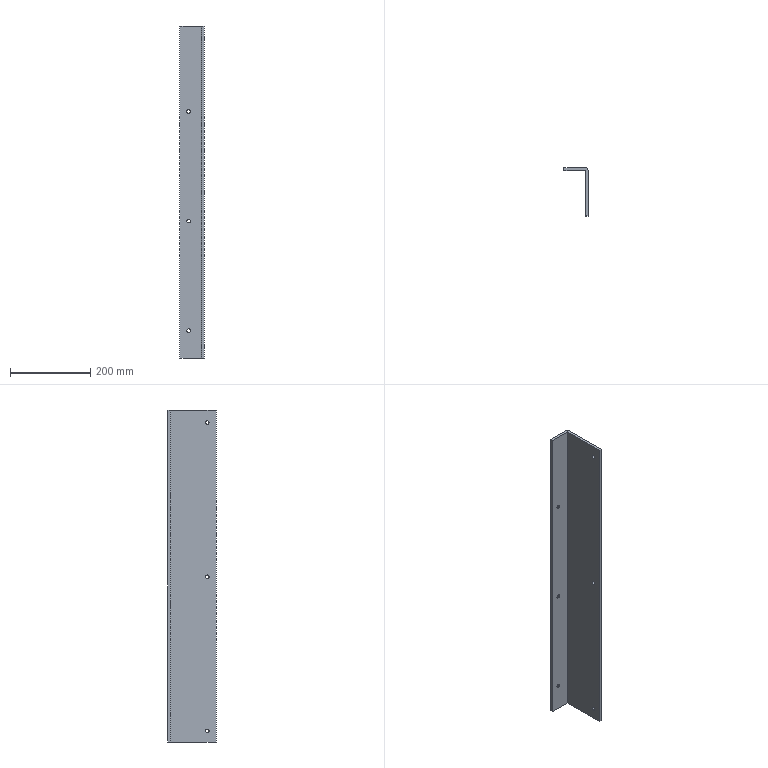Part | SolidWorks | features BaseBody 1 | 1 solid | 28 faces | box 60 x 120 x 827 mm | volume 851995 mm3 | cylinder 14 | plane 8 | cone 6 | commonest cylinder face diameters 9 x12 1.473 x1 13.473 x1
STEP:
#1=CARTESIAN_POINT('',(-6.,22.,800.));
#2=VERTEX_POINT('',#1);
#3=CARTESIAN_POINT('',(-6.,22.,791.));
#4=VERTEX_POINT('',#3);
#5=CARTESIAN_POINT('',(-6.,22.,795.5));
#6=DIRECTION('',(1.,0.,0.));
#7=DIRECTION('',(0.,0.,-1.));
#8=AXIS2_PLACEMENT_3D('',#5,#6,#7);
#9=CIRCLE('',#8,4.5);
#10=EDGE_CURVE('',#2,#4,#9,.T.);
#11=ORIENTED_EDGE('',*,*,#10,.F.);
#12=CARTESIAN_POINT('',(0.,22.,800.));
#13=VERTEX_POINT('',#12);
#14=CARTESIAN_POINT('',(-60.,22.,800.));
#15=DIRECTION('',(1.,0.,0.));
#16=VECTOR('',#15,1000.);
#17=LINE('',#14,#16);
#18=EDGE_CURVE('',#2,#13,#17,.T.);
#19=ORIENTED_EDGE('',*,*,#18,.T.);
#20=CARTESIAN_POINT('',(0.,22.,791.));
#21=VERTEX_POINT('',#20);
#22=CARTESIAN_POINT('',(0.,22.,795.5));
#23=DIRECTION('',(1.,0.,0.));
#24=DIRECTION('',(0.,0.,-1.));
#25=AXIS2_PLACEMENT_3D('',#22,#23,#24);
#26=CIRCLE('',#25,4.5);
#27=EDGE_CURVE('',#13,#21,#26,.T.);
#28=ORIENTED_EDGE('',*,*,#27,.T.);
#29=CARTESIAN_POINT('',(-60.,22.,791.));
#30=DIRECTION('',(1.,0.,0.));
#31=VECTOR('',#30,1000.);
#32=LINE('',#29,#31);
#33=EDGE_CURVE('',#4,#21,#32,.T.);
#34=ORIENTED_EDGE('',*,*,#33,.F.);
#35=EDGE_LOOP('',(#11,#19,#28,#34));
#36=FACE_OUTER_BOUND('',#35,.T.);
#37=CARTESIAN_POINT('',(-60.,22.,795.5));
#38=DIRECTION('',(1.,0.,0.));
#39=DIRECTION('',(0.,0.,-1.));
#40=AXIS2_PLACEMENT_3D('',#37,#38,#39);
#41=CYLINDRICAL_SURFACE('',#40,4.5);
#42=ADVANCED_FACE('',(#36),#41,.F.);
#43=CARTESIAN_POINT('',(-6.,22.,416.));
#44=VERTEX_POINT('',#43);
#45=CARTESIAN_POINT('',(-6.,22.,407.));
#46=VERTEX_POINT('',#45);
#47=CARTESIAN_POINT('',(-6.,22.,411.5));
#48=DIRECTION('',(1.,0.,0.));
#49=DIRECTION('',(0.,0.,-1.));
#50=AXIS2_PLACEMENT_3D('',#47,#48,#49);
#51=CIRCLE('',#50,4.5);
#52=EDGE_CURVE('',#44,#46,#51,.T.);
#53=ORIENTED_EDGE('',*,*,#52,.F.);
#54=CARTESIAN_POINT('',(0.,22.,416.));
#55=VERTEX_POINT('',#54);
#56=CARTESIAN_POINT('',(-60.,22.,416.));
#57=DIRECTION('',(1.,0.,0.));
#58=VECTOR('',#57,1000.);
#59=LINE('',#56,#58);
#60=EDGE_CURVE('',#44,#55,#59,.T.);
#61=ORIENTED_EDGE('',*,*,#60,.T.);
#62=CARTESIAN_POINT('',(0.,22.,407.));
#63=VERTEX_POINT('',#62);
#64=CARTESIAN_POINT('',(0.,22.,411.5));
#65=DIRECTION('',(1.,0.,0.));
#66=DIRECTION('',(0.,0.,-1.));
#67=AXIS2_PLACEMENT_3D('',#64,#65,#66);
#68=CIRCLE('',#67,4.5);
#69=EDGE_CURVE('',#55,#63,#68,.T.);
#70=ORIENTED_EDGE('',*,*,#69,.T.);
#71=CARTESIAN_POINT('',(-60.,22.,407.));
#72=DIRECTION('',(1.,0.,0.));
#73=VECTOR('',#72,1000.);
#74=LINE('',#71,#73);
#75=EDGE_CURVE('',#46,#63,#74,.T.);
#76=ORIENTED_EDGE('',*,*,#75,.F.);
#77=EDGE_LOOP('',(#53,#61,#70,#76));
#78=FACE_OUTER_BOUND('',#77,.T.);
#79=CARTESIAN_POINT('',(-60.,22.,411.5));
#80=DIRECTION('',(1.,0.,0.));
#81=DIRECTION('',(0.,0.,-1.));
#82=AXIS2_PLACEMENT_3D('',#79,#80,#81);
#83=CYLINDRICAL_SURFACE('',#82,4.5);
#84=ADVANCED_FACE('',(#78),#83,.F.);
#85=CARTESIAN_POINT('',(-6.,22.,32.));
#86=VERTEX_POINT('',#85);
#87=CARTESIAN_POINT('',(-6.,22.,23.));
#88=VERTEX_POINT('',#87);
#89=CARTESIAN_POINT('',(-6.,22.,27.5));
#90=DIRECTION('',(1.,0.,0.));
#91=DIRECTION('',(0.,0.,-1.));
#92=AXIS2_PLACEMENT_3D('',#89,#90,#91);
#93=CIRCLE('',#92,4.5);
#94=EDGE_CURVE('',#86,#88,#93,.T.);
#95=ORIENTED_EDGE('',*,*,#94,.F.);
#96=CARTESIAN_POINT('',(0.,22.,32.));
#97=VERTEX_POINT('',#96);
#98=CARTESIAN_POINT('',(-60.,22.,32.));
#99=DIRECTION('',(1.,0.,0.));
#100=VECTOR('',#99,1000.);
#101=LINE('',#98,#100);
#102=EDGE_CURVE('',#86,#97,#101,.T.);
#103=ORIENTED_EDGE('',*,*,#102,.T.);
#104=CARTESIAN_POINT('',(0.,22.,23.));
#105=VERTEX_POINT('',#104);
#106=CARTESIAN_POINT('',(0.,22.,27.5));
#107=DIRECTION('',(1.,0.,0.));
#108=DIRECTION('',(0.,0.,-1.));
#109=AXIS2_PLACEMENT_3D('',#106,#107,#108);
#110=CIRCLE('',#109,4.5);
#111=EDGE_CURVE('',#97,#105,#110,.T.);
#112=ORIENTED_EDGE('',*,*,#111,.T.);
#113=CARTESIAN_POINT('',(-60.,22.,23.));
#114=DIRECTION('',(1.,0.,0.));
#115=VECTOR('',#114,1000.);
#116=LINE('',#113,#115);
#117=EDGE_CURVE('',#88,#105,#116,.T.);
#118=ORIENTED_EDGE('',*,*,#117,.F.);
#119=EDGE_LOOP('',(#95,#103,#112,#118));
#120=FACE_OUTER_BOUND('',#119,.T.);
#121=CARTESIAN_POINT('',(-60.,22.,27.5));
#122=DIRECTION('',(1.,0.,0.));
#123=DIRECTION('',(0.,0.,-1.));
#124=AXIS2_PLACEMENT_3D('',#121,#122,#123);
#125=CYLINDRICAL_SURFACE('',#124,4.5);
#126=ADVANCED_FACE('',(#120),#125,.F.);
#127=CARTESIAN_POINT('',(-34.,115.5,68.));
#128=VERTEX_POINT('',#127);
#129=CARTESIAN_POINT('',(-38.5,115.5,63.5));
#130=VERTEX_POINT('',#129);
#131=CARTESIAN_POINT('',(-38.5,115.5,68.));
#132=DIRECTION('',(0.,1.,0.));
#133=DIRECTION('',(0.,0.,1.));
#134=AXIS2_PLACEMENT_3D('',#131,#132,#133);
#135=CIRCLE('',#134,4.5);
#136=EDGE_CURVE('',#128,#130,#135,.T.);
#137=ORIENTED_EDGE('',*,*,#136,.F.);
#138=CARTESIAN_POINT('',(-29.5,120.,68.));
#139=VERTEX_POINT('',#138);
#140=CARTESIAN_POINT('',(-29.5,120.,68.));
#141=DIRECTION('',(0.7071,0.7071,0.));
#142=VECTOR('',#141,1000.);
#143=LINE('',#140,#142);
#144=EDGE_CURVE('',#128,#139,#143,.T.);
#145=ORIENTED_EDGE('',*,*,#144,.T.);
#146=CARTESIAN_POINT('',(-47.5,120.,68.));
#147=VERTEX_POINT('',#146);
#148=CARTESIAN_POINT('',(-38.5,120.,68.));
#149=DIRECTION('',(0.,1.,0.));
#150=DIRECTION('',(-1.,0.,0.));
#151=AXIS2_PLACEMENT_3D('',#148,#149,#150);
#152=CIRCLE('',#151,9.);
#153=EDGE_CURVE('',#139,#147,#152,.T.);
#154=ORIENTED_EDGE('',*,*,#153,.T.);
#155=CARTESIAN_POINT('',(-43.,115.5,68.));
#156=VERTEX_POINT('',#155);
#157=CARTESIAN_POINT('',(-47.5,120.,68.));
#158=DIRECTION('',(-0.7071,0.7071,0.));
#159=VECTOR('',#158,1000.);
#160=LINE('',#157,#159);
#161=EDGE_CURVE('',#156,#147,#160,.T.);
#162=ORIENTED_EDGE('',*,*,#161,.F.);
#163=CARTESIAN_POINT('',(-38.5,115.5,68.));
#164=DIRECTION('',(0.,1.,0.));
#165=DIRECTION('',(0.,0.,1.));
#166=AXIS2_PLACEMENT_3D('',#163,#164,#165);
#167=CIRCLE('',#166,4.5);
#168=EDGE_CURVE('',#130,#156,#167,.T.);
#169=ORIENTED_EDGE('',*,*,#168,.F.);
#170=EDGE_LOOP('',(#137,#145,#154,#162,#169));
#171=FACE_OUTER_BOUND('',#170,.T.);
#172=CARTESIAN_POINT('',(-38.5,120.,68.));
#173=DIRECTION('',(0.,1.,0.));
#174=DIRECTION('',(-1.,0.,0.));
#175=AXIS2_PLACEMENT_3D('',#172,#173,#174);
#176=CONICAL_SURFACE('',#175,9.,0.7854);
#177=ADVANCED_FACE('',(#171),#176,.F.);
#178=CARTESIAN_POINT('',(-34.,115.5,614.));
#179=VERTEX_POINT('',#178);
#180=CARTESIAN_POINT('',(-38.5,115.5,609.5));
#181=VERTEX_POINT('',#180);
#182=CARTESIAN_POINT('',(-38.5,115.5,614.));
#183=DIRECTION('',(0.,1.,0.));
#184=DIRECTION('',(0.,0.,1.));
#185=AXIS2_PLACEMENT_3D('',#182,#183,#184);
#186=CIRCLE('',#185,4.5);
#187=EDGE_CURVE('',#179,#181,#186,.T.);
#188=ORIENTED_EDGE('',*,*,#187,.F.);
#189=CARTESIAN_POINT('',(-29.5,120.,614.));
#190=VERTEX_POINT('',#189);
#191=CARTESIAN_POINT('',(-29.5,120.,614.));
#192=DIRECTION('',(0.7071,0.7071,0.));
#193=VECTOR('',#192,1000.);
#194=LINE('',#191,#193);
#195=EDGE_CURVE('',#179,#190,#194,.T.);
#196=ORIENTED_EDGE('',*,*,#195,.T.);
#197=CARTESIAN_POINT('',(-47.5,120.,614.));
#198=VERTEX_POINT('',#197);
#199=CARTESIAN_POINT('',(-38.5,120.,614.));
#200=DIRECTION('',(0.,1.,0.));
#201=DIRECTION('',(-1.,0.,0.));
#202=AXIS2_PLACEMENT_3D('',#199,#200,#201);
#203=CIRCLE('',#202,9.);
#204=EDGE_CURVE('',#190,#198,#203,.T.);
#205=ORIENTED_EDGE('',*,*,#204,.T.);
#206=CARTESIAN_POINT('',(-43.,115.5,614.));
#207=VERTEX_POINT('',#206);
#208=CARTESIAN_POINT('',(-47.5,120.,614.));
#209=DIRECTION('',(-0.7071,0.7071,0.));
#210=VECTOR('',#209,1000.);
#211=LINE('',#208,#210);
#212=EDGE_CURVE('',#207,#198,#211,.T.);
#213=ORIENTED_EDGE('',*,*,#212,.F.);
#214=CARTESIAN_POINT('',(-38.5,115.5,614.));
#215=DIRECTION('',(0.,1.,0.));
#216=DIRECTION('',(0.,0.,1.));
#217=AXIS2_PLACEMENT_3D('',#214,#215,#216);
#218=CIRCLE('',#217,4.5);
#219=EDGE_CURVE('',#181,#207,#218,.T.);
#220=ORIENTED_EDGE('',*,*,#219,.F.);
#221=EDGE_LOOP('',(#188,#196,#205,#213,#220));
#222=FACE_OUTER_BOUND('',#221,.T.);
#223=CARTESIAN_POINT('',(-38.5,120.,614.));
#224=DIRECTION('',(0.,1.,0.));
#225=DIRECTION('',(-1.,0.,0.));
#226=AXIS2_PLACEMENT_3D('',#223,#224,#225);
#227=CONICAL_SURFACE('',#226,9.,0.7854);
#228=ADVANCED_FACE('',(#222),#227,.F.);
#229=CARTESIAN_POINT('',(-34.,115.5,341.));
#230=VERTEX_POINT('',#229);
#231=CARTESIAN_POINT('',(-38.5,115.5,336.5));
#232=VERTEX_POINT('',#231);
#233=CARTESIAN_POINT('',(-38.5,115.5,341.));
#234=DIRECTION('',(0.,1.,0.));
#235=DIRECTION('',(0.,0.,1.));
#236=AXIS2_PLACEMENT_3D('',#233,#234,#235);
#237=CIRCLE('',#236,4.5);
#238=EDGE_CURVE('',#230,#232,#237,.T.);
#239=ORIENTED_EDGE('',*,*,#238,.F.);
#240=CARTESIAN_POINT('',(-29.5,120.,341.));
#241=VERTEX_POINT('',#240);
#242=CARTESIAN_POINT('',(-29.5,120.,341.));
#243=DIRECTION('',(0.7071,0.7071,0.));
#244=VECTOR('',#243,1000.);
#245=LINE('',#242,#244);
#246=EDGE_CURVE('',#230,#241,#245,.T.);
#247=ORIENTED_EDGE('',*,*,#246,.T.);
#248=CARTESIAN_POINT('',(-47.5,120.,341.));
#249=VERTEX_POINT('',#248);
#250=CARTESIAN_POINT('',(-38.5,120.,341.));
#251=DIRECTION('',(0.,1.,0.));
#252=DIRECTION('',(-1.,0.,0.));
#253=AXIS2_PLACEMENT_3D('',#250,#251,#252);
#254=CIRCLE('',#253,9.);
#255=EDGE_CURVE('',#241,#249,#254,.T.);
#256=ORIENTED_EDGE('',*,*,#255,.T.);
#257=CARTESIAN_POINT('',(-43.,115.5,341.));
#258=VERTEX_POINT('',#257);
#259=CARTESIAN_POINT('',(-47.5,120.,341.));
#260=DIRECTION('',(-0.7071,0.7071,0.));
#261=VECTOR('',#260,1000.);
#262=LINE('',#259,#261);
#263=EDGE_CURVE('',#258,#249,#262,.T.);
#264=ORIENTED_EDGE('',*,*,#263,.F.);
#265=CARTESIAN_POINT('',(-38.5,115.5,341.));
#266=DIRECTION('',(0.,1.,0.));
#267=DIRECTION('',(0.,0.,1.));
#268=AXIS2_PLACEMENT_3D('',#265,#266,#267);
#269=CIRCLE('',#268,4.5);
#270=EDGE_CURVE('',#232,#258,#269,.T.);
#271=ORIENTED_EDGE('',*,*,#270,.F.);
#272=EDGE_LOOP('',(#239,#247,#256,#264,#271));
#273=FACE_OUTER_BOUND('',#272,.T.);
#274=CARTESIAN_POINT('',(-38.5,120.,341.));
#275=DIRECTION('',(0.,1.,0.));
#276=DIRECTION('',(-1.,0.,0.));
#277=AXIS2_PLACEMENT_3D('',#274,#275,#276);
#278=CONICAL_SURFACE('',#277,9.,0.7854);
#279=ADVANCED_FACE('',(#273),#278,.F.);
#280=CARTESIAN_POINT('',(-38.5,114.,63.5));
#281=VERTEX_POINT('',#280);
#282=CARTESIAN_POINT('',(-38.5,114.,72.5));
#283=VERTEX_POINT('',#282);
#284=CARTESIAN_POINT('',(-38.5,114.,68.));
#285=DIRECTION('',(0.,1.,0.));
#286=DIRECTION('',(0.,0.,1.));
#287=AXIS2_PLACEMENT_3D('',#284,#285,#286);
#288=CIRCLE('',#287,4.5);
#289=EDGE_CURVE('',#281,#283,#288,.T.);
#290=ORIENTED_EDGE('',*,*,#289,.F.);
#291=CARTESIAN_POINT('',(-38.5,120.,63.5));
#292=DIRECTION('',(0.,1.,0.));
#293=VECTOR('',#292,1000.);
#294=LINE('',#291,#293);
#295=EDGE_CURVE('',#281,#130,#294,.T.);
#296=ORIENTED_EDGE('',*,*,#295,.T.);
#297=ORIENTED_EDGE('',*,*,#168,.T.);
#298=CARTESIAN_POINT('',(-38.5,115.5,72.5));
#299=VERTEX_POINT('',#298);
#300=CARTESIAN_POINT('',(-38.5,115.5,68.));
#301=DIRECTION('',(0.,1.,0.));
#302=DIRECTION('',(0.,0.,1.));
#303=AXIS2_PLACEMENT_3D('',#300,#301,#302);
#304=CIRCLE('',#303,4.5);
#305=EDGE_CURVE('',#156,#299,#304,.T.);
#306=ORIENTED_EDGE('',*,*,#305,.T.);
#307=CARTESIAN_POINT('',(-38.5,120.,72.5));
#308=DIRECTION('',(0.,1.,0.));
#309=VECTOR('',#308,1000.);
#310=LINE('',#307,#309);
#311=EDGE_CURVE('',#283,#299,#310,.T.);
#312=ORIENTED_EDGE('',*,*,#311,.F.);
#313=EDGE_LOOP('',(#290,#296,#297,#306,#312));
#314=FACE_OUTER_BOUND('',#313,.T.);
#315=CARTESIAN_POINT('',(-38.5,120.,68.));
#316=DIRECTION('',(0.,1.,0.));
#317=DIRECTION('',(0.,0.,1.));
#318=AXIS2_PLACEMENT_3D('',#315,#316,#317);
#319=CYLINDRICAL_SURFACE('',#318,4.5);
#320=ADVANCED_FACE('',(#314),#319,.F.);
#321=CARTESIAN_POINT('',(-38.5,114.,609.5));
#322=VERTEX_POINT('',#321);
#323=CARTESIAN_POINT('',(-38.5,114.,618.5));
#324=VERTEX_POINT('',#323);
#325=CARTESIAN_POINT('',(-38.5,114.,614.));
#326=DIRECTION('',(0.,1.,0.));
#327=DIRECTION('',(0.,0.,1.));
#328=AXIS2_PLACEMENT_3D('',#325,#326,#327);
#329=CIRCLE('',#328,4.5);
#330=EDGE_CURVE('',#322,#324,#329,.T.);
#331=ORIENTED_EDGE('',*,*,#330,.F.);
#332=CARTESIAN_POINT('',(-38.5,120.,609.5));
#333=DIRECTION('',(0.,1.,0.));
#334=VECTOR('',#333,1000.);
#335=LINE('',#332,#334);
#336=EDGE_CURVE('',#322,#181,#335,.T.);
#337=ORIENTED_EDGE('',*,*,#336,.T.);
#338=ORIENTED_EDGE('',*,*,#219,.T.);
#339=CARTESIAN_POINT('',(-38.5,115.5,618.5));
#340=VERTEX_POINT('',#339);
#341=CARTESIAN_POINT('',(-38.5,115.5,614.));
#342=DIRECTION('',(0.,1.,0.));
#343=DIRECTION('',(0.,0.,1.));
#344=AXIS2_PLACEMENT_3D('',#341,#342,#343);
#345=CIRCLE('',#344,4.5);
#346=EDGE_CURVE('',#207,#340,#345,.T.);
#347=ORIENTED_EDGE('',*,*,#346,.T.);
#348=CARTESIAN_POINT('',(-38.5,120.,618.5));
#349=DIRECTION('',(0.,1.,0.));
#350=VECTOR('',#349,1000.);
#351=LINE('',#348,#350);
#352=EDGE_CURVE('',#324,#340,#351,.T.);
#353=ORIENTED_EDGE('',*,*,#352,.F.);
#354=EDGE_LOOP('',(#331,#337,#338,#347,#353));
#355=FACE_OUTER_BOUND('',#354,.T.);
#356=CARTESIAN_POINT('',(-38.5,120.,614.));
#357=DIRECTION('',(0.,1.,0.));
#358=DIRECTION('',(0.,0.,1.));
#359=AXIS2_PLACEMENT_3D('',#356,#357,#358);
#360=CYLINDRICAL_SURFACE('',#359,4.5);
#361=ADVANCED_FACE('',(#355),#360,.F.);
#362=CARTESIAN_POINT('',(-38.5,114.,336.5));
#363=VERTEX_POINT('',#362);
#364=CARTESIAN_POINT('',(-38.5,114.,345.5));
#365=VERTEX_POINT('',#364);
#366=CARTESIAN_POINT('',(-38.5,114.,341.));
#367=DIRECTION('',(0.,1.,0.));
#368=DIRECTION('',(0.,0.,1.));
#369=AXIS2_PLACEMENT_3D('',#366,#367,#368);
#370=CIRCLE('',#369,4.5);
#371=EDGE_CURVE('',#363,#365,#370,.T.);
#372=ORIENTED_EDGE('',*,*,#371,.F.);
#373=CARTESIAN_POINT('',(-38.5,120.,336.5));
#374=DIRECTION('',(0.,1.,0.));
#375=VECTOR('',#374,1000.);
#376=LINE('',#373,#375);
#377=EDGE_CURVE('',#363,#232,#376,.T.);
#378=ORIENTED_EDGE('',*,*,#377,.T.);
#379=ORIENTED_EDGE('',*,*,#270,.T.);
#380=CARTESIAN_POINT('',(-38.5,115.5,345.5));
#381=VERTEX_POINT('',#380);
#382=CARTESIAN_POINT('',(-38.5,115.5,341.));
#383=DIRECTION('',(0.,1.,0.));
#384=DIRECTION('',(0.,0.,1.));
#385=AXIS2_PLACEMENT_3D('',#382,#383,#384);
#386=CIRCLE('',#385,4.5);
#387=EDGE_CURVE('',#258,#381,#386,.T.);
#388=ORIENTED_EDGE('',*,*,#387,.T.);
#389=CARTESIAN_POINT('',(-38.5,120.,345.5));
#390=DIRECTION('',(0.,1.,0.));
#391=VECTOR('',#390,1000.);
#392=LINE('',#389,#391);
#393=EDGE_CURVE('',#365,#381,#392,.T.);
#394=ORIENTED_EDGE('',*,*,#393,.F.);
#395=EDGE_LOOP('',(#372,#378,#379,#388,#394));
#396=FACE_OUTER_BOUND('',#395,.T.);
#397=CARTESIAN_POINT('',(-38.5,120.,341.));
#398=DIRECTION('',(0.,1.,0.));
#399=DIRECTION('',(0.,0.,1.));
#400=AXIS2_PLACEMENT_3D('',#397,#398,#399);
#401=CYLINDRICAL_SURFACE('',#400,4.5);
#402=ADVANCED_FACE('',(#396),#401,.F.);
#403=CARTESIAN_POINT('',(0.,113.263,827.));
#404=VERTEX_POINT('',#403);
#405=CARTESIAN_POINT('',(0.,113.263,0.));
#406=VERTEX_POINT('',#405);
#407=CARTESIAN_POINT('',(0.,113.263,827.));
#408=DIRECTION('',(0.,0.,-1.));
#409=VECTOR('',#408,1000.);
#410=LINE('',#407,#409);
#411=EDGE_CURVE('',#404,#406,#410,.T.);
#412=ORIENTED_EDGE('',*,*,#411,.F.);
#413=CARTESIAN_POINT('',(0.,0.,827.));
#414=VERTEX_POINT('',#413);
#415=CARTESIAN_POINT('',(0.,0.,827.));
#416=DIRECTION('',(0.,1.,0.));
#417=VECTOR('',#416,1000.);
#418=LINE('',#415,#417);
#419=EDGE_CURVE('',#414,#404,#418,.T.);
#420=ORIENTED_EDGE('',*,*,#419,.F.);
#421=CARTESIAN_POINT('',(0.,0.,0.));
#422=VERTEX_POINT('',#421);
#423=CARTESIAN_POINT('',(0.,0.,827.));
#424=DIRECTION('',(0.,0.,1.));
#425=VECTOR('',#424,1000.);
#426=LINE('',#423,#425);
#427=EDGE_CURVE('',#422,#414,#426,.T.);
#428=ORIENTED_EDGE('',*,*,#427,.F.);
#429=CARTESIAN_POINT('',(0.,0.,0.));
#430=DIRECTION('',(0.,-1.,0.));
#431=VECTOR('',#430,1000.);
#432=LINE('',#429,#431);
#433=EDGE_CURVE('',#406,#422,#432,.T.);
#434=ORIENTED_EDGE('',*,*,#433,.F.);
#435=EDGE_LOOP('',(#412,#420,#428,#434));
#436=FACE_OUTER_BOUND('',#435,.T.);
#437=CARTESIAN_POINT('',(0.,22.,795.5));
#438=DIRECTION('',(1.,0.,0.));
#439=DIRECTION('',(0.,0.,-1.));
#440=AXIS2_PLACEMENT_3D('',#437,#438,#439);
#441=CIRCLE('',#440,4.5);
#442=EDGE_CURVE('',#21,#13,#441,.T.);
#443=ORIENTED_EDGE('',*,*,#442,.F.);
#444=ORIENTED_EDGE('',*,*,#27,.F.);
#445=EDGE_LOOP('',(#443,#444));
#446=FACE_BOUND('',#445,.T.);
#447=CARTESIAN_POINT('',(0.,22.,411.5));
#448=DIRECTION('',(1.,0.,0.));
#449=DIRECTION('',(0.,0.,-1.));
#450=AXIS2_PLACEMENT_3D('',#447,#448,#449);
#451=CIRCLE('',#450,4.5);
#452=EDGE_CURVE('',#63,#55,#451,.T.);
#453=ORIENTED_EDGE('',*,*,#452,.F.);
#454=ORIENTED_EDGE('',*,*,#69,.F.);
#455=EDGE_LOOP('',(#453,#454));
#456=FACE_BOUND('',#455,.T.);
#457=CARTESIAN_POINT('',(0.,22.,27.5));
#458=DIRECTION('',(1.,0.,0.));
#459=DIRECTION('',(0.,0.,-1.));
#460=AXIS2_PLACEMENT_3D('',#457,#458,#459);
#461=CIRCLE('',#460,4.5);
#462=EDGE_CURVE('',#105,#97,#461,.T.);
#463=ORIENTED_EDGE('',*,*,#462,.F.);
#464=ORIENTED_EDGE('',*,*,#111,.F.);
#465=EDGE_LOOP('',(#463,#464));
#466=FACE_BOUND('',#465,.T.);
#467=CARTESIAN_POINT('',(0.,0.,827.));
#468=DIRECTION('',(-1.,0.,0.));
#469=DIRECTION('',(0.,0.,1.));
#470=AXIS2_PLACEMENT_3D('',#467,#468,#469);
#471=PLANE('',#470);
#472=ADVANCED_FACE('',(#436,#446,#456,#466),#471,.F.);
#473=CARTESIAN_POINT('',(-6.,113.263,0.));
#474=VERTEX_POINT('',#473);
#475=CARTESIAN_POINT('',(-6.,0.,0.));
#476=VERTEX_POINT('',#475);
#477=CARTESIAN_POINT('',(-6.,113.263,0.));
#478=DIRECTION('',(0.,-1.,0.));
#479=VECTOR('',#478,1000.);
#480=LINE('',#477,#479);
#481=EDGE_CURVE('',#474,#476,#480,.T.);
#482=ORIENTED_EDGE('',*,*,#481,.F.);
#483=CARTESIAN_POINT('',(-6.737,114.,0.));
#484=VERTEX_POINT('',#483);
#485=CARTESIAN_POINT('',(-6.737,113.263,0.));
#486=DIRECTION('',(0.,0.,1.));
#487=DIRECTION('',(-1.,0.,0.));
#488=AXIS2_PLACEMENT_3D('',#485,#486,#487);
#489=CIRCLE('',#488,0.7366);
#490=EDGE_CURVE('',#474,#484,#489,.T.);
#491=ORIENTED_EDGE('',*,*,#490,.T.);
#492=CARTESIAN_POINT('',(-60.,114.,0.));
#493=VERTEX_POINT('',#492);
#494=CARTESIAN_POINT('',(-6.,114.,0.));
#495=DIRECTION('',(-1.,0.,0.));
#496=VECTOR('',#495,1000.);
#497=LINE('',#494,#496);
#498=EDGE_CURVE('',#484,#493,#497,.T.);
#499=ORIENTED_EDGE('',*,*,#498,.T.);
#500=CARTESIAN_POINT('',(-60.,120.,0.));
#501=VERTEX_POINT('',#500);
#502=CARTESIAN_POINT('',(-60.,113.263,0.));
#503=DIRECTION('',(0.,1.,0.));
#504=VECTOR('',#503,1000.);
#505=LINE('',#502,#504);
#506=EDGE_CURVE('',#493,#501,#505,.T.);
#507=ORIENTED_EDGE('',*,*,#506,.T.);
#508=CARTESIAN_POINT('',(-6.737,120.,0.));
#509=VERTEX_POINT('',#508);
#510=CARTESIAN_POINT('',(0.,120.,0.));
#511=DIRECTION('',(1.,0.,0.));
#512=VECTOR('',#511,1000.);
#513=LINE('',#510,#512);
#514=EDGE_CURVE('',#501,#509,#513,.T.);
#515=ORIENTED_EDGE('',*,*,#514,.T.);
#516=CARTESIAN_POINT('',(-6.737,113.263,0.));
#517=DIRECTION('',(0.,0.,1.));
#518=DIRECTION('',(-1.,0.,0.));
#519=AXIS2_PLACEMENT_3D('',#516,#517,#518);
#520=CIRCLE('',#519,6.737);
#521=EDGE_CURVE('',#406,#509,#520,.T.);
#522=ORIENTED_EDGE('',*,*,#521,.F.);
#523=ORIENTED_EDGE('',*,*,#433,.T.);
#524=CARTESIAN_POINT('',(-6.737,0.,0.));
#525=DIRECTION('',(1.,0.,0.));
#526=VECTOR('',#525,1000.);
#527=LINE('',#524,#526);
#528=EDGE_CURVE('',#476,#422,#527,.T.);
#529=ORIENTED_EDGE('',*,*,#528,.F.);
#530=EDGE_LOOP('',(#482,#491,#499,#507,#515,#522,#523,#529));
#531=FACE_OUTER_BOUND('',#530,.T.);
#532=CARTESIAN_POINT('',(-6.737,113.263,0.));
#533=DIRECTION('',(0.,0.,1.));
#534=DIRECTION('',(1.,0.,0.));
#535=AXIS2_PLACEMENT_3D('',#532,#533,#534);
#536=PLANE('',#535);
#537=ADVANCED_FACE('',(#531),#536,.F.);
#538=CARTESIAN_POINT('',(-6.737,120.,827.));
#539=VERTEX_POINT('',#538);
#540=CARTESIAN_POINT('',(-6.737,113.263,827.));
#541=DIRECTION('',(0.,0.,-1.));
#542=DIRECTION('',(-1.,0.,0.));
#543=AXIS2_PLACEMENT_3D('',#540,#541,#542);
#544=CIRCLE('',#543,6.737);
#545=EDGE_CURVE('',#539,#404,#544,.T.);
#546=ORIENTED_EDGE('',*,*,#545,.T.);
#547=ORIENTED_EDGE('',*,*,#411,.T.);
#548=ORIENTED_EDGE('',*,*,#521,.T.);
#549=CARTESIAN_POINT('',(-6.737,120.,827.));
#550=DIRECTION('',(0.,0.,1.));
#551=VECTOR('',#550,1000.);
#552=LINE('',#549,#551);
#553=EDGE_CURVE('',#509,#539,#552,.T.);
#554=ORIENTED_EDGE('',*,*,#553,.T.);
#555=EDGE_LOOP('',(#546,#547,#548,#554));
#556=FACE_OUTER_BOUND('',#555,.T.);
#557=CARTESIAN_POINT('',(-6.737,113.263,827.));
#558=DIRECTION('',(0.,0.,-1.));
#559=DIRECTION('',(-1.,0.,0.));
#560=AXIS2_PLACEMENT_3D('',#557,#558,#559);
#561=CYLINDRICAL_SURFACE('',#560,6.737);
#562=ADVANCED_FACE('',(#556),#561,.T.);
#563=CARTESIAN_POINT('',(-6.,113.263,827.));
#564=VERTEX_POINT('',#563);
#565=CARTESIAN_POINT('',(-6.,0.,827.));
#566=VERTEX_POINT('',#565);
#567=CARTESIAN_POINT('',(-6.,114.,827.));
#568=DIRECTION('',(0.,-1.,0.));
#569=VECTOR('',#568,1000.);
#570=LINE('',#567,#569);
#571=EDGE_CURVE('',#564,#566,#570,.T.);
#572=ORIENTED_EDGE('',*,*,#571,.T.);
#573=CARTESIAN_POINT('',(-6.737,0.,827.));
#574=DIRECTION('',(1.,0.,0.));
#575=VECTOR('',#574,1000.);
#576=LINE('',#573,#575);
#577=EDGE_CURVE('',#566,#414,#576,.T.);
#578=ORIENTED_EDGE('',*,*,#577,.T.);
#579=ORIENTED_EDGE('',*,*,#419,.T.);
#580=ORIENTED_EDGE('',*,*,#545,.F.);
#581=CARTESIAN_POINT('',(-60.,120.,827.));
#582=VERTEX_POINT('',#581);
#583=CARTESIAN_POINT('',(0.,120.,827.));
#584=DIRECTION('',(-1.,0.,0.));
#585=VECTOR('',#584,1000.);
#586=LINE('',#583,#585);
#587=EDGE_CURVE('',#539,#582,#586,.T.);
#588=ORIENTED_EDGE('',*,*,#587,.T.);
#589=CARTESIAN_POINT('',(-60.,114.,827.));
#590=VERTEX_POINT('',#589);
#591=CARTESIAN_POINT('',(-60.,113.263,827.));
#592=DIRECTION('',(0.,-1.,0.));
#593=VECTOR('',#592,1000.);
#594=LINE('',#591,#593);
#595=EDGE_CURVE('',#582,#590,#594,.T.);
#596=ORIENTED_EDGE('',*,*,#595,.T.);
#597=CARTESIAN_POINT('',(-6.737,114.,827.));
#598=VERTEX_POINT('',#597);
#599=CARTESIAN_POINT('',(-6.737,114.,827.));
#600=DIRECTION('',(1.,0.,0.));
#601=VECTOR('',#600,1000.);
#602=LINE('',#599,#601);
#603=EDGE_CURVE('',#590,#598,#602,.T.);
#604=ORIENTED_EDGE('',*,*,#603,.T.);
#605=CARTESIAN_POINT('',(-6.737,113.263,827.));
#606=DIRECTION('',(0.,0.,-1.));
#607=DIRECTION('',(-1.,0.,0.));
#608=AXIS2_PLACEMENT_3D('',#605,#606,#607);
#609=CIRCLE('',#608,0.7366);
#610=EDGE_CURVE('',#598,#564,#609,.T.);
#611=ORIENTED_EDGE('',*,*,#610,.T.);
#612=EDGE_LOOP('',(#572,#578,#579,#580,#588,#596,#604,#611));
#613=FACE_OUTER_BOUND('',#612,.T.);
#614=CARTESIAN_POINT('',(-6.737,114.,827.));
#615=DIRECTION('',(0.,0.,1.));
#616=DIRECTION('',(1.,0.,0.));
#617=AXIS2_PLACEMENT_3D('',#614,#615,#616);
#618=PLANE('',#617);
#619=ADVANCED_FACE('',(#613),#618,.T.);
#620=ORIENTED_EDGE('',*,*,#577,.F.);
#621=CARTESIAN_POINT('',(-6.,0.,827.));
#622=DIRECTION('',(0.,0.,-1.));
#623=VECTOR('',#622,1000.);
#624=LINE('',#621,#623);
#625=EDGE_CURVE('',#566,#476,#624,.T.);
#626=ORIENTED_EDGE('',*,*,#625,.T.);
#627=ORIENTED_EDGE('',*,*,#528,.T.);
#628=ORIENTED_EDGE('',*,*,#427,.T.);
#629=EDGE_LOOP('',(#620,#626,#627,#628));
#630=FACE_OUTER_BOUND('',#629,.T.);
#631=CARTESIAN_POINT('',(0.,0.,827.));
#632=DIRECTION('',(0.,-1.,0.));
#633=DIRECTION('',(0.,0.,-1.));
#634=AXIS2_PLACEMENT_3D('',#631,#632,#633);
#635=PLANE('',#634);
#636=ADVANCED_FACE('',(#630),#635,.T.);
#637=ORIENTED_EDGE('',*,*,#18,.F.);
#638=CARTESIAN_POINT('',(-6.,22.,795.5));
#639=DIRECTION('',(1.,0.,0.));
#640=DIRECTION('',(0.,0.,-1.));
#641=AXIS2_PLACEMENT_3D('',#638,#639,#640);
#642=CIRCLE('',#641,4.5);
#643=EDGE_CURVE('',#4,#2,#642,.T.);
#644=ORIENTED_EDGE('',*,*,#643,.F.);
#645=ORIENTED_EDGE('',*,*,#33,.T.);
#646=ORIENTED_EDGE('',*,*,#442,.T.);
#647=EDGE_LOOP('',(#637,#644,#645,#646));
#648=FACE_OUTER_BOUND('',#647,.T.);
#649=CARTESIAN_POINT('',(-60.,22.,795.5));
#650=DIRECTION('',(1.,0.,0.));
#651=DIRECTION('',(0.,0.,-1.));
#652=AXIS2_PLACEMENT_3D('',#649,#650,#651);
#653=CYLINDRICAL_SURFACE('',#652,4.5);
#654=ADVANCED_FACE('',(#648),#653,.F.);
#655=ORIENTED_EDGE('',*,*,#60,.F.);
#656=CARTESIAN_POINT('',(-6.,22.,411.5));
#657=DIRECTION('',(1.,0.,0.));
#658=DIRECTION('',(0.,0.,-1.));
#659=AXIS2_PLACEMENT_3D('',#656,#657,#658);
#660=CIRCLE('',#659,4.5);
#661=EDGE_CURVE('',#46,#44,#660,.T.);
#662=ORIENTED_EDGE('',*,*,#661,.F.);
#663=ORIENTED_EDGE('',*,*,#75,.T.);
#664=ORIENTED_EDGE('',*,*,#452,.T.);
#665=EDGE_LOOP('',(#655,#662,#663,#664));
#666=FACE_OUTER_BOUND('',#665,.T.);
#667=CARTESIAN_POINT('',(-60.,22.,411.5));
#668=DIRECTION('',(1.,0.,0.));
#669=DIRECTION('',(0.,0.,-1.));
#670=AXIS2_PLACEMENT_3D('',#667,#668,#669);
#671=CYLINDRICAL_SURFACE('',#670,4.5);
#672=ADVANCED_FACE('',(#666),#671,.F.);
#673=ORIENTED_EDGE('',*,*,#102,.F.);
#674=CARTESIAN_POINT('',(-6.,22.,27.5));
#675=DIRECTION('',(1.,0.,0.));
#676=DIRECTION('',(0.,0.,-1.));
#677=AXIS2_PLACEMENT_3D('',#674,#675,#676);
#678=CIRCLE('',#677,4.5);
#679=EDGE_CURVE('',#88,#86,#678,.T.);
#680=ORIENTED_EDGE('',*,*,#679,.F.);
#681=ORIENTED_EDGE('',*,*,#117,.T.);
#682=ORIENTED_EDGE('',*,*,#462,.T.);
#683=EDGE_LOOP('',(#673,#680,#681,#682));
#684=FACE_OUTER_BOUND('',#683,.T.);
#685=CARTESIAN_POINT('',(-60.,22.,27.5));
#686=DIRECTION('',(1.,0.,0.));
#687=DIRECTION('',(0.,0.,-1.));
#688=AXIS2_PLACEMENT_3D('',#685,#686,#687);
#689=CYLINDRICAL_SURFACE('',#688,4.5);
#690=ADVANCED_FACE('',(#684),#689,.F.);
#691=ORIENTED_EDGE('',*,*,#571,.F.);
#692=CARTESIAN_POINT('',(-6.,113.263,827.));
#693=DIRECTION('',(0.,0.,-1.));
#694=VECTOR('',#693,1000.);
#695=LINE('',#692,#694);
#696=EDGE_CURVE('',#564,#474,#695,.T.);
#697=ORIENTED_EDGE('',*,*,#696,.T.);
#698=ORIENTED_EDGE('',*,*,#481,.T.);
#699=ORIENTED_EDGE('',*,*,#625,.F.);
#700=EDGE_LOOP('',(#691,#697,#698,#699));
#701=FACE_OUTER_BOUND('',#700,.T.);
#702=ORIENTED_EDGE('',*,*,#643,.T.);
#703=ORIENTED_EDGE('',*,*,#10,.T.);
#704=EDGE_LOOP('',(#702,#703));
#705=FACE_BOUND('',#704,.T.);
#706=ORIENTED_EDGE('',*,*,#661,.T.);
#707=ORIENTED_EDGE('',*,*,#52,.T.);
#708=EDGE_LOOP('',(#706,#707));
#709=FACE_BOUND('',#708,.T.);
#710=ORIENTED_EDGE('',*,*,#679,.T.);
#711=ORIENTED_EDGE('',*,*,#94,.T.);
#712=EDGE_LOOP('',(#710,#711));
#713=FACE_BOUND('',#712,.T.);
#714=CARTESIAN_POINT('',(-6.,0.,827.));
#715=DIRECTION('',(-1.,0.,0.));
#716=DIRECTION('',(0.,0.,1.));
#717=AXIS2_PLACEMENT_3D('',#714,#715,#716);
#718=PLANE('',#717);
#719=ADVANCED_FACE('',(#701,#705,#709,#713),#718,.T.);
#720=CARTESIAN_POINT('',(-38.5,120.,68.));
#721=DIRECTION('',(0.,1.,0.));
#722=DIRECTION('',(-1.,0.,0.));
#723=AXIS2_PLACEMENT_3D('',#720,#721,#722);
#724=CIRCLE('',#723,9.);
#725=EDGE_CURVE('',#147,#139,#724,.T.);
#726=ORIENTED_EDGE('',*,*,#725,.F.);
#727=ORIENTED_EDGE('',*,*,#153,.F.);
#728=EDGE_LOOP('',(#726,#727));
#729=FACE_BOUND('',#728,.T.);
#730=CARTESIAN_POINT('',(-38.5,120.,614.));
#731=DIRECTION('',(0.,1.,0.));
#732=DIRECTION('',(-1.,0.,0.));
#733=AXIS2_PLACEMENT_3D('',#730,#731,#732);
#734=CIRCLE('',#733,9.);
#735=EDGE_CURVE('',#198,#190,#734,.T.);
#736=ORIENTED_EDGE('',*,*,#735,.F.);
#737=ORIENTED_EDGE('',*,*,#204,.F.);
#738=EDGE_LOOP('',(#736,#737));
#739=FACE_BOUND('',#738,.T.);
#740=CARTESIAN_POINT('',(-60.,120.,827.));
#741=DIRECTION('',(0.,0.,-1.));
#742=VECTOR('',#741,1000.);
#743=LINE('',#740,#742);
#744=EDGE_CURVE('',#582,#501,#743,.T.);
#745=ORIENTED_EDGE('',*,*,#744,.F.);
#746=ORIENTED_EDGE('',*,*,#587,.F.);
#747=ORIENTED_EDGE('',*,*,#553,.F.);
#748=ORIENTED_EDGE('',*,*,#514,.F.);
#749=EDGE_LOOP('',(#745,#746,#747,#748));
#750=FACE_OUTER_BOUND('',#749,.T.);
#751=CARTESIAN_POINT('',(-38.5,120.,341.));
#752=DIRECTION('',(0.,1.,0.));
#753=DIRECTION('',(-1.,0.,0.));
#754=AXIS2_PLACEMENT_3D('',#751,#752,#753);
#755=CIRCLE('',#754,9.);
#756=EDGE_CURVE('',#249,#241,#755,.T.);
#757=ORIENTED_EDGE('',*,*,#756,.F.);
#758=ORIENTED_EDGE('',*,*,#255,.F.);
#759=EDGE_LOOP('',(#757,#758));
#760=FACE_BOUND('',#759,.T.);
#761=CARTESIAN_POINT('',(0.,120.,827.));
#762=DIRECTION('',(0.,-1.,0.));
#763=DIRECTION('',(0.,0.,-1.));
#764=AXIS2_PLACEMENT_3D('',#761,#762,#763);
#765=PLANE('',#764);
#766=ADVANCED_FACE('',(#729,#739,#750,#760),#765,.F.);
#767=ORIENTED_EDGE('',*,*,#696,.F.);
#768=ORIENTED_EDGE('',*,*,#610,.F.);
#769=CARTESIAN_POINT('',(-6.737,114.,827.));
#770=DIRECTION('',(0.,0.,1.));
#771=VECTOR('',#770,1000.);
#772=LINE('',#769,#771);
#773=EDGE_CURVE('',#484,#598,#772,.T.);
#774=ORIENTED_EDGE('',*,*,#773,.F.);
#775=ORIENTED_EDGE('',*,*,#490,.F.);
#776=EDGE_LOOP('',(#767,#768,#774,#775));
#777=FACE_OUTER_BOUND('',#776,.T.);
#778=CARTESIAN_POINT('',(-6.737,113.263,827.));
#779=DIRECTION('',(0.,0.,-1.));
#780=DIRECTION('',(-1.,0.,0.));
#781=AXIS2_PLACEMENT_3D('',#778,#779,#780);
#782=CYLINDRICAL_SURFACE('',#781,0.7366);
#783=ADVANCED_FACE('',(#777),#782,.F.);
#784=ORIENTED_EDGE('',*,*,#144,.F.);
#785=CARTESIAN_POINT('',(-38.5,115.5,68.));
#786=DIRECTION('',(0.,1.,0.));
#787=DIRECTION('',(0.,0.,1.));
#788=AXIS2_PLACEMENT_3D('',#785,#786,#787);
#789=CIRCLE('',#788,4.5);
#790=EDGE_CURVE('',#299,#128,#789,.T.);
#791=ORIENTED_EDGE('',*,*,#790,.F.);
#792=ORIENTED_EDGE('',*,*,#305,.F.);
#793=ORIENTED_EDGE('',*,*,#161,.T.);
#794=ORIENTED_EDGE('',*,*,#725,.T.);
#795=EDGE_LOOP('',(#784,#791,#792,#793,#794));
#796=FACE_OUTER_BOUND('',#795,.T.);
#797=CARTESIAN_POINT('',(-38.5,120.,68.));
#798=DIRECTION('',(0.,1.,0.));
#799=DIRECTION('',(-1.,0.,0.));
#800=AXIS2_PLACEMENT_3D('',#797,#798,#799);
#801=CONICAL_SURFACE('',#800,9.,0.7854);
#802=ADVANCED_FACE('',(#796),#801,.F.);
#803=ORIENTED_EDGE('',*,*,#195,.F.);
#804=CARTESIAN_POINT('',(-38.5,115.5,614.));
#805=DIRECTION('',(0.,1.,0.));
#806=DIRECTION('',(0.,0.,1.));
#807=AXIS2_PLACEMENT_3D('',#804,#805,#806);
#808=CIRCLE('',#807,4.5);
#809=EDGE_CURVE('',#340,#179,#808,.T.);
#810=ORIENTED_EDGE('',*,*,#809,.F.);
#811=ORIENTED_EDGE('',*,*,#346,.F.);
#812=ORIENTED_EDGE('',*,*,#212,.T.);
#813=ORIENTED_EDGE('',*,*,#735,.T.);
#814=EDGE_LOOP('',(#803,#810,#811,#812,#813));
#815=FACE_OUTER_BOUND('',#814,.T.);
#816=CARTESIAN_POINT('',(-38.5,120.,614.));
#817=DIRECTION('',(0.,1.,0.));
#818=DIRECTION('',(-1.,0.,0.));
#819=AXIS2_PLACEMENT_3D('',#816,#817,#818);
#820=CONICAL_SURFACE('',#819,9.,0.7854);
#821=ADVANCED_FACE('',(#815),#820,.F.);
#822=ORIENTED_EDGE('',*,*,#595,.F.);
#823=ORIENTED_EDGE('',*,*,#744,.T.);
#824=ORIENTED_EDGE('',*,*,#506,.F.);
#825=CARTESIAN_POINT('',(-60.,114.,827.));
#826=DIRECTION('',(0.,0.,1.));
#827=VECTOR('',#826,1000.);
#828=LINE('',#825,#827);
#829=EDGE_CURVE('',#493,#590,#828,.T.);
#830=ORIENTED_EDGE('',*,*,#829,.T.);
#831=EDGE_LOOP('',(#822,#823,#824,#830));
#832=FACE_OUTER_BOUND('',#831,.T.);
#833=CARTESIAN_POINT('',(-60.,114.,827.));
#834=DIRECTION('',(-1.,0.,0.));
#835=DIRECTION('',(0.,0.,1.));
#836=AXIS2_PLACEMENT_3D('',#833,#834,#835);
#837=PLANE('',#836);
#838=ADVANCED_FACE('',(#832),#837,.T.);
#839=ORIENTED_EDGE('',*,*,#246,.F.);
#840=CARTESIAN_POINT('',(-38.5,115.5,341.));
#841=DIRECTION('',(0.,1.,0.));
#842=DIRECTION('',(0.,0.,1.));
#843=AXIS2_PLACEMENT_3D('',#840,#841,#842);
#844=CIRCLE('',#843,4.5);
#845=EDGE_CURVE('',#381,#230,#844,.T.);
#846=ORIENTED_EDGE('',*,*,#845,.F.);
#847=ORIENTED_EDGE('',*,*,#387,.F.);
#848=ORIENTED_EDGE('',*,*,#263,.T.);
#849=ORIENTED_EDGE('',*,*,#756,.T.);
#850=EDGE_LOOP('',(#839,#846,#847,#848,#849));
#851=FACE_OUTER_BOUND('',#850,.T.);
#852=CARTESIAN_POINT('',(-38.5,120.,341.));
#853=DIRECTION('',(0.,1.,0.));
#854=DIRECTION('',(-1.,0.,0.));
#855=AXIS2_PLACEMENT_3D('',#852,#853,#854);
#856=CONICAL_SURFACE('',#855,9.,0.7854);
#857=ADVANCED_FACE('',(#851),#856,.F.);
#858=CARTESIAN_POINT('',(-38.5,114.,68.));
#859=DIRECTION('',(0.,1.,0.));
#860=DIRECTION('',(0.,0.,1.));
#861=AXIS2_PLACEMENT_3D('',#858,#859,#860);
#862=CIRCLE('',#861,4.5);
#863=EDGE_CURVE('',#283,#281,#862,.T.);
#864=ORIENTED_EDGE('',*,*,#863,.T.);
#865=ORIENTED_EDGE('',*,*,#289,.T.);
#866=EDGE_LOOP('',(#864,#865));
#867=FACE_BOUND('',#866,.T.);
#868=ORIENTED_EDGE('',*,*,#603,.F.);
#869=ORIENTED_EDGE('',*,*,#829,.F.);
#870=ORIENTED_EDGE('',*,*,#498,.F.);
#871=ORIENTED_EDGE('',*,*,#773,.T.);
#872=EDGE_LOOP('',(#868,#869,#870,#871));
#873=FACE_OUTER_BOUND('',#872,.T.);
#874=CARTESIAN_POINT('',(-38.5,114.,614.));
#875=DIRECTION('',(0.,1.,0.));
#876=DIRECTION('',(0.,0.,1.));
#877=AXIS2_PLACEMENT_3D('',#874,#875,#876);
#878=CIRCLE('',#877,4.5);
#879=EDGE_CURVE('',#324,#322,#878,.T.);
#880=ORIENTED_EDGE('',*,*,#879,.T.);
#881=ORIENTED_EDGE('',*,*,#330,.T.);
#882=EDGE_LOOP('',(#880,#881));
#883=FACE_BOUND('',#882,.T.);
#884=CARTESIAN_POINT('',(-38.5,114.,341.));
#885=DIRECTION('',(0.,1.,0.));
#886=DIRECTION('',(0.,0.,1.));
#887=AXIS2_PLACEMENT_3D('',#884,#885,#886);
#888=CIRCLE('',#887,4.5);
#889=EDGE_CURVE('',#365,#363,#888,.T.);
#890=ORIENTED_EDGE('',*,*,#889,.T.);
#891=ORIENTED_EDGE('',*,*,#371,.T.);
#892=EDGE_LOOP('',(#890,#891));
#893=FACE_BOUND('',#892,.T.);
#894=CARTESIAN_POINT('',(0.,114.,827.));
#895=DIRECTION('',(0.,-1.,0.));
#896=DIRECTION('',(0.,0.,-1.));
#897=AXIS2_PLACEMENT_3D('',#894,#895,#896);
#898=PLANE('',#897);
#899=ADVANCED_FACE('',(#867,#873,#883,#893),#898,.T.);
#900=ORIENTED_EDGE('',*,*,#295,.F.);
#901=ORIENTED_EDGE('',*,*,#863,.F.);
#902=ORIENTED_EDGE('',*,*,#311,.T.);
#903=ORIENTED_EDGE('',*,*,#790,.T.);
#904=ORIENTED_EDGE('',*,*,#136,.T.);
#905=EDGE_LOOP('',(#900,#901,#902,#903,#904));
#906=FACE_OUTER_BOUND('',#905,.T.);
#907=CARTESIAN_POINT('',(-38.5,120.,68.));
#908=DIRECTION('',(0.,1.,0.));
#909=DIRECTION('',(0.,0.,1.));
#910=AXIS2_PLACEMENT_3D('',#907,#908,#909);
#911=CYLINDRICAL_SURFACE('',#910,4.5);
#912=ADVANCED_FACE('',(#906),#911,.F.);
#913=ORIENTED_EDGE('',*,*,#336,.F.);
#914=ORIENTED_EDGE('',*,*,#879,.F.);
#915=ORIENTED_EDGE('',*,*,#352,.T.);
#916=ORIENTED_EDGE('',*,*,#809,.T.);
#917=ORIENTED_EDGE('',*,*,#187,.T.);
#918=EDGE_LOOP('',(#913,#914,#915,#916,#917));
#919=FACE_OUTER_BOUND('',#918,.T.);
#920=CARTESIAN_POINT('',(-38.5,120.,614.));
#921=DIRECTION('',(0.,1.,0.));
#922=DIRECTION('',(0.,0.,1.));
#923=AXIS2_PLACEMENT_3D('',#920,#921,#922);
#924=CYLINDRICAL_SURFACE('',#923,4.5);
#925=ADVANCED_FACE('',(#919),#924,.F.);
#926=ORIENTED_EDGE('',*,*,#377,.F.);
#927=ORIENTED_EDGE('',*,*,#889,.F.);
#928=ORIENTED_EDGE('',*,*,#393,.T.);
#929=ORIENTED_EDGE('',*,*,#845,.T.);
#930=ORIENTED_EDGE('',*,*,#238,.T.);
#931=EDGE_LOOP('',(#926,#927,#928,#929,#930));
#932=FACE_OUTER_BOUND('',#931,.T.);
#933=CARTESIAN_POINT('',(-38.5,120.,341.));
#934=DIRECTION('',(0.,1.,0.));
#935=DIRECTION('',(0.,0.,1.));
#936=AXIS2_PLACEMENT_3D('',#933,#934,#935);
#937=CYLINDRICAL_SURFACE('',#936,4.5);
#938=ADVANCED_FACE('',(#932),#937,.F.);
#939=CLOSED_SHELL('',(#42,#84,#126,#177,#228,#279,#320,#361,#402,#472,#537,#562,#619,#636,#654,#672,#690,#719,#766,#783,#802,#821,#838,#857,#899,#912,#925,#938));
#940=MANIFOLD_SOLID_BREP('',#939);
#941=CARTESIAN_POINT('',(0.,0.,0.));
#942=DIRECTION('',(0.,0.,1.));
#943=DIRECTION('',(1.,0.,0.));
#944=AXIS2_PLACEMENT_3D('',#941,#942,#943);
#945=(LENGTH_UNIT()NAMED_UNIT(*)SI_UNIT(.MILLI.,.METRE.));
#946=UNCERTAINTY_MEASURE_WITH_UNIT(LENGTH_MEASURE(0.00001),#945,'','');
#947=(NAMED_UNIT(*)PLANE_ANGLE_UNIT()SI_UNIT($,.RADIAN.));
#948=(NAMED_UNIT(*)SI_UNIT($,.STERADIAN.)SOLID_ANGLE_UNIT());
#949=(GEOMETRIC_REPRESENTATION_CONTEXT(3)GLOBAL_UNCERTAINTY_ASSIGNED_CONTEXT((#946))GLOBAL_UNIT_ASSIGNED_CONTEXT((#945,#947,#948))REPRESENTATION_CONTEXT('',''));
#950=ADVANCED_BREP_SHAPE_REPRESENTATION('',(#940,#944),#949);